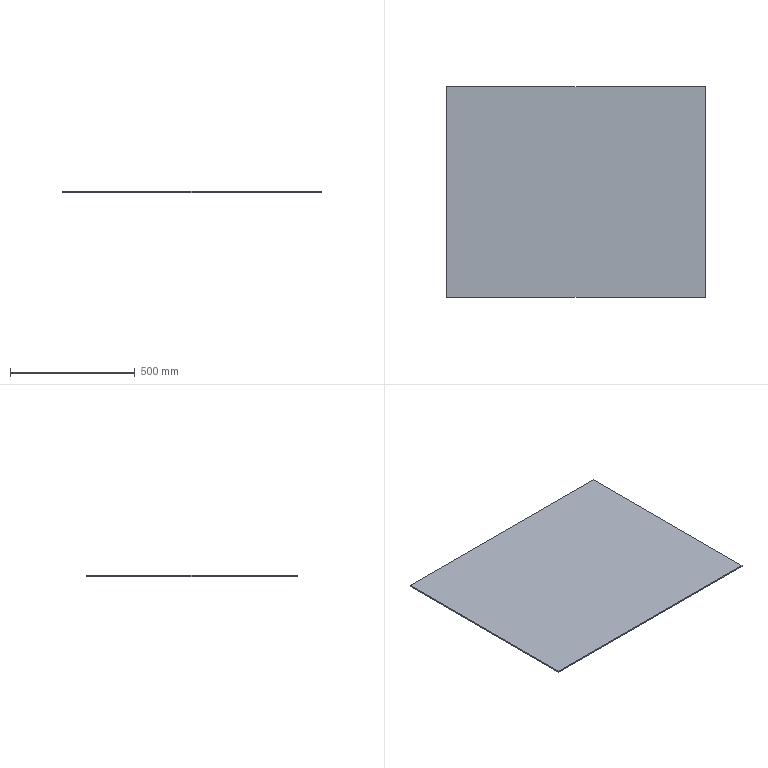Part | SolidWorks | features Extrusion 1, HoleWzd 1 | 1 solid | 6 faces | box 1037 x 843 x 5 mm | volume 4370955 mm3 | plane 6
STEP:
#1=CARTESIAN_POINT('',(518.5,-421.5,0.));
#2=VERTEX_POINT('',#1);
#3=CARTESIAN_POINT('',(518.5,421.5,0.));
#4=VERTEX_POINT('',#3);
#5=CARTESIAN_POINT('',(518.5,421.5,0.));
#6=DIRECTION('',(0.,1.,0.));
#7=VECTOR('',#6,1000.);
#8=LINE('',#5,#7);
#9=EDGE_CURVE('',#2,#4,#8,.T.);
#10=ORIENTED_EDGE('',*,*,#9,.T.);
#11=CARTESIAN_POINT('',(518.5,421.5,5.));
#12=VERTEX_POINT('',#11);
#13=CARTESIAN_POINT('',(518.5,421.5,5.));
#14=DIRECTION('',(0.,0.,-1.));
#15=VECTOR('',#14,1000.);
#16=LINE('',#13,#15);
#17=EDGE_CURVE('',#12,#4,#16,.T.);
#18=ORIENTED_EDGE('',*,*,#17,.F.);
#19=CARTESIAN_POINT('',(518.5,-421.5,5.));
#20=VERTEX_POINT('',#19);
#21=CARTESIAN_POINT('',(518.5,421.5,5.));
#22=DIRECTION('',(0.,1.,0.));
#23=VECTOR('',#22,1000.);
#24=LINE('',#21,#23);
#25=EDGE_CURVE('',#20,#12,#24,.T.);
#26=ORIENTED_EDGE('',*,*,#25,.F.);
#27=CARTESIAN_POINT('',(518.5,-421.5,5.));
#28=DIRECTION('',(0.,0.,-1.));
#29=VECTOR('',#28,1000.);
#30=LINE('',#27,#29);
#31=EDGE_CURVE('',#20,#2,#30,.T.);
#32=ORIENTED_EDGE('',*,*,#31,.T.);
#33=EDGE_LOOP('',(#10,#18,#26,#32));
#34=FACE_OUTER_BOUND('',#33,.T.);
#35=CARTESIAN_POINT('',(518.5,421.5,5.));
#36=DIRECTION('',(-1.,0.,0.));
#37=DIRECTION('',(0.,0.,1.));
#38=AXIS2_PLACEMENT_3D('',#35,#36,#37);
#39=PLANE('',#38);
#40=ADVANCED_FACE('',(#34),#39,.F.);
#41=CARTESIAN_POINT('',(-518.5,421.5,0.));
#42=VERTEX_POINT('',#41);
#43=CARTESIAN_POINT('',(-518.5,421.5,0.));
#44=DIRECTION('',(-1.,0.,0.));
#45=VECTOR('',#44,1000.);
#46=LINE('',#43,#45);
#47=EDGE_CURVE('',#4,#42,#46,.T.);
#48=ORIENTED_EDGE('',*,*,#47,.T.);
#49=CARTESIAN_POINT('',(-518.5,421.5,5.));
#50=VERTEX_POINT('',#49);
#51=CARTESIAN_POINT('',(-518.5,421.5,5.));
#52=DIRECTION('',(0.,0.,-1.));
#53=VECTOR('',#52,1000.);
#54=LINE('',#51,#53);
#55=EDGE_CURVE('',#50,#42,#54,.T.);
#56=ORIENTED_EDGE('',*,*,#55,.F.);
#57=CARTESIAN_POINT('',(-518.5,421.5,5.));
#58=DIRECTION('',(-1.,0.,0.));
#59=VECTOR('',#58,1000.);
#60=LINE('',#57,#59);
#61=EDGE_CURVE('',#12,#50,#60,.T.);
#62=ORIENTED_EDGE('',*,*,#61,.F.);
#63=ORIENTED_EDGE('',*,*,#17,.T.);
#64=EDGE_LOOP('',(#48,#56,#62,#63));
#65=FACE_OUTER_BOUND('',#64,.T.);
#66=CARTESIAN_POINT('',(-518.5,421.5,5.));
#67=DIRECTION('',(0.,-1.,0.));
#68=DIRECTION('',(0.,0.,-1.));
#69=AXIS2_PLACEMENT_3D('',#66,#67,#68);
#70=PLANE('',#69);
#71=ADVANCED_FACE('',(#65),#70,.F.);
#72=CARTESIAN_POINT('',(-518.5,-421.5,0.));
#73=VERTEX_POINT('',#72);
#74=CARTESIAN_POINT('',(-518.5,421.5,0.));
#75=DIRECTION('',(0.,-1.,0.));
#76=VECTOR('',#75,1000.);
#77=LINE('',#74,#76);
#78=EDGE_CURVE('',#42,#73,#77,.T.);
#79=ORIENTED_EDGE('',*,*,#78,.T.);
#80=CARTESIAN_POINT('',(-518.5,-421.5,5.));
#81=VERTEX_POINT('',#80);
#82=CARTESIAN_POINT('',(-518.5,-421.5,5.));
#83=DIRECTION('',(0.,0.,-1.));
#84=VECTOR('',#83,1000.);
#85=LINE('',#82,#84);
#86=EDGE_CURVE('',#81,#73,#85,.T.);
#87=ORIENTED_EDGE('',*,*,#86,.F.);
#88=CARTESIAN_POINT('',(-518.5,421.5,5.));
#89=DIRECTION('',(0.,-1.,0.));
#90=VECTOR('',#89,1000.);
#91=LINE('',#88,#90);
#92=EDGE_CURVE('',#50,#81,#91,.T.);
#93=ORIENTED_EDGE('',*,*,#92,.F.);
#94=ORIENTED_EDGE('',*,*,#55,.T.);
#95=EDGE_LOOP('',(#79,#87,#93,#94));
#96=FACE_OUTER_BOUND('',#95,.T.);
#97=CARTESIAN_POINT('',(-518.5,421.5,5.));
#98=DIRECTION('',(1.,0.,0.));
#99=DIRECTION('',(0.,1.,0.));
#100=AXIS2_PLACEMENT_3D('',#97,#98,#99);
#101=PLANE('',#100);
#102=ADVANCED_FACE('',(#96),#101,.F.);
#103=CARTESIAN_POINT('',(-518.5,-421.5,0.));
#104=DIRECTION('',(1.,0.,0.));
#105=VECTOR('',#104,1000.);
#106=LINE('',#103,#105);
#107=EDGE_CURVE('',#73,#2,#106,.T.);
#108=ORIENTED_EDGE('',*,*,#107,.T.);
#109=ORIENTED_EDGE('',*,*,#31,.F.);
#110=CARTESIAN_POINT('',(-518.5,-421.5,5.));
#111=DIRECTION('',(1.,0.,0.));
#112=VECTOR('',#111,1000.);
#113=LINE('',#110,#112);
#114=EDGE_CURVE('',#81,#20,#113,.T.);
#115=ORIENTED_EDGE('',*,*,#114,.F.);
#116=ORIENTED_EDGE('',*,*,#86,.T.);
#117=EDGE_LOOP('',(#108,#109,#115,#116));
#118=FACE_OUTER_BOUND('',#117,.T.);
#119=CARTESIAN_POINT('',(-518.5,-421.5,5.));
#120=DIRECTION('',(0.,1.,0.));
#121=DIRECTION('',(0.,0.,1.));
#122=AXIS2_PLACEMENT_3D('',#119,#120,#121);
#123=PLANE('',#122);
#124=ADVANCED_FACE('',(#118),#123,.F.);
#125=ORIENTED_EDGE('',*,*,#25,.T.);
#126=ORIENTED_EDGE('',*,*,#61,.T.);
#127=ORIENTED_EDGE('',*,*,#92,.T.);
#128=ORIENTED_EDGE('',*,*,#114,.T.);
#129=EDGE_LOOP('',(#125,#126,#127,#128));
#130=FACE_OUTER_BOUND('',#129,.T.);
#131=CARTESIAN_POINT('',(0.,0.,5.));
#132=DIRECTION('',(0.,0.,1.));
#133=DIRECTION('',(1.,0.,0.));
#134=AXIS2_PLACEMENT_3D('',#131,#132,#133);
#135=PLANE('',#134);
#136=ADVANCED_FACE('',(#130),#135,.T.);
#137=ORIENTED_EDGE('',*,*,#9,.F.);
#138=ORIENTED_EDGE('',*,*,#107,.F.);
#139=ORIENTED_EDGE('',*,*,#78,.F.);
#140=ORIENTED_EDGE('',*,*,#47,.F.);
#141=EDGE_LOOP('',(#137,#138,#139,#140));
#142=FACE_OUTER_BOUND('',#141,.T.);
#143=CARTESIAN_POINT('',(0.,0.,0.));
#144=DIRECTION('',(0.,0.,1.));
#145=DIRECTION('',(1.,0.,0.));
#146=AXIS2_PLACEMENT_3D('',#143,#144,#145);
#147=PLANE('',#146);
#148=ADVANCED_FACE('',(#142),#147,.F.);
#149=CLOSED_SHELL('',(#40,#71,#102,#124,#136,#148));
#150=MANIFOLD_SOLID_BREP('',#149);
#151=CARTESIAN_POINT('',(0.,0.,0.));
#152=DIRECTION('',(0.,0.,1.));
#153=DIRECTION('',(1.,0.,0.));
#154=AXIS2_PLACEMENT_3D('',#151,#152,#153);
#155=(LENGTH_UNIT()NAMED_UNIT(*)SI_UNIT(.MILLI.,.METRE.));
#156=UNCERTAINTY_MEASURE_WITH_UNIT(LENGTH_MEASURE(0.00001),#155,'','');
#157=(NAMED_UNIT(*)PLANE_ANGLE_UNIT()SI_UNIT($,.RADIAN.));
#158=(NAMED_UNIT(*)SI_UNIT($,.STERADIAN.)SOLID_ANGLE_UNIT());
#159=(GEOMETRIC_REPRESENTATION_CONTEXT(3)GLOBAL_UNCERTAINTY_ASSIGNED_CONTEXT((#156))GLOBAL_UNIT_ASSIGNED_CONTEXT((#155,#157,#158))REPRESENTATION_CONTEXT('',''));
#160=ADVANCED_BREP_SHAPE_REPRESENTATION('',(#150,#154),#159);